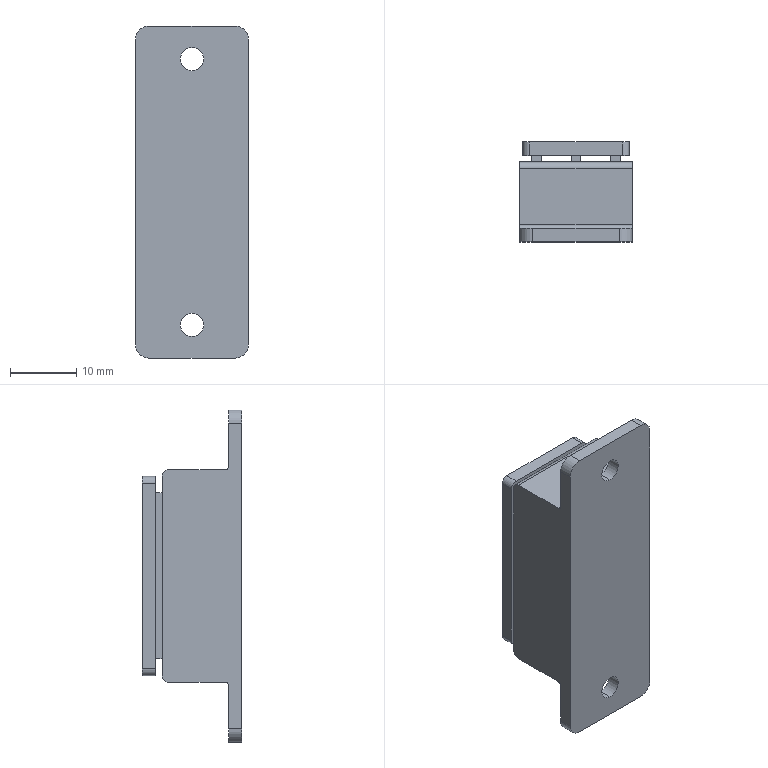Part | SolidWorks | features BaseBody 1 | 1 solid | 54 faces | box 17 x 15 x 50 mm | volume 8082 mm3 | plane 30 | cylinder 20 | cone 4 | commonest cylinder face diameters 2 x6 3.5 x4 4 x4 4.2 x4 1 x2